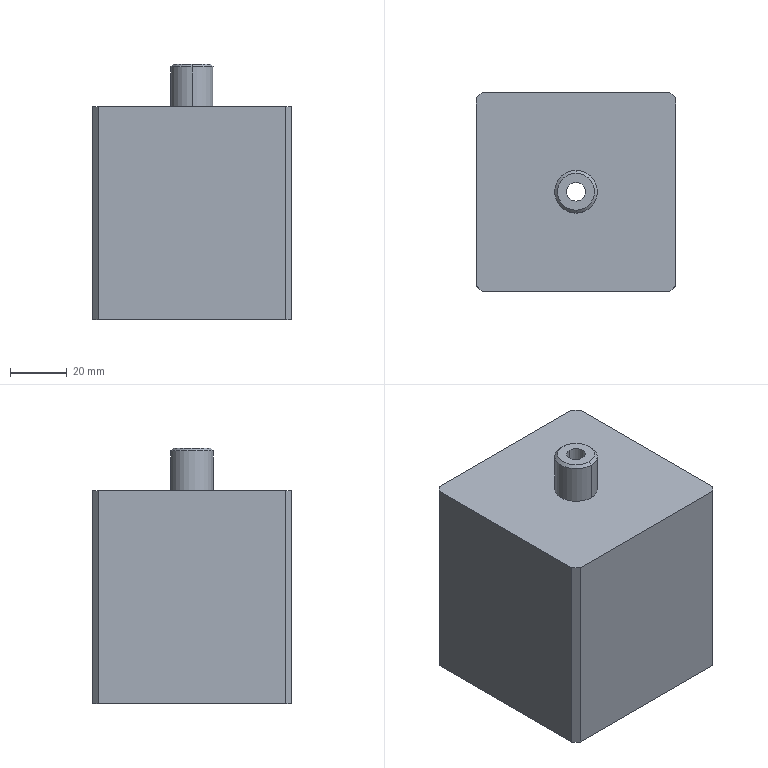NC program | NX | posted with a generic post | part box 70 x 70 x 90 mm
Lines 7860 to 8019 of 10206:
(ZLEVEL_PROFILE_COPY_COPY , TOOL : D10)
N15706 T04 M6
N15708 G54
N15710 G17 G0 G90 X-15.583 Y10.337 S7500 M3
N15712 G43 Z30. H4
N15714 Z-8.214
N15716 G94 G1 Z-9.714 F1000.
N15718 X-17.225 Y10.843
N15720 G3 X-18.2 Y10.62 R1.
N15722 G1 Y-10.62 F850.
N15724 G3 X18.2 Y-10.62 R25.64
N15726 G1 Y10.62
N15728 G3 X-18.2 Y10.62 R25.64
N15730 X-17.7 Y9.754 R1.
N15732 G1 X-16.2 Y8.888
N15734 Z-8.214
N15736 G0 X-15.583 Y10.337 Z-17.929
N15738 G1 Z-19.429 F1000.
N15740 X-17.225 Y10.843
N15742 G3 X-18.2 Y10.62 R1.
N15744 G1 Y-10.62 F850.
N15746 G3 X18.2 Y-10.62 R25.64
N15748 G1 Y10.62
N15750 G3 X-18.2 Y10.62 R25.64
N15752 X-17.7 Y9.754 R1.
N15754 G1 X-16.2 Y8.888
N15756 Z-17.929
N15758 G0 X-15.583 Y10.337 Z-27.643
N15760 G1 Z-29.143 F1000.
N15762 X-17.225 Y10.843
N15764 G3 X-18.2 Y10.62 R1.
N15766 G1 Y-10.621 F850.
N15768 G3 X18.2 Y-10.621 R25.64
N15770 G1 Y10.62
N15772 G3 X-18.2 Y10.62 R25.64
N15774 X-17.7 Y9.754 R1.
N15776 G1 X-16.2 Y8.888
N15778 Z-27.643
N15780 G0 X-15.583 Y10.337 Z-37.357
N15782 G1 Z-38.857 F1000.
N15784 X-17.225 Y10.843
N15786 G3 X-18.2 Y10.62 R1.
N15788 G1 Y-10.621 F850.
N15790 G3 X18.2 Y-10.621 R25.64
N15792 G1 Y10.62
N15794 G3 X-18.2 Y10.62 R25.64
N15796 X-17.7 Y9.754 R1.
N15798 G1 X-16.2 Y8.888
N15800 Z-37.357
N15802 G0 X-15.583 Y10.337 Z-47.071
N15804 G1 Z-48.571 F1000.
N15806 X-17.225 Y10.843
N15808 G3 X-18.2 Y10.62 R1.
N15810 G1 Y-10.621 F850.
N15812 G3 X18.2 Y-10.621 R25.64
N15814 G1 Y10.62
N15816 G3 X-18.2 Y10.62 R25.64
N15818 X-17.7 Y9.754 R1.
N15820 G1 X-16.2 Y8.888
N15822 Z-47.071
N15824 G0 X-15.583 Y10.337 Z-56.786
N15826 G1 Z-58.286 F1000.
N15828 X-17.225 Y10.843
N15830 G3 X-18.2 Y10.62 R1.
N15832 G1 Y-10.621 F850.
N15834 G3 X18.2 Y-10.621 R25.64
N15836 G1 Y10.62
N15838 G3 X-18.2 Y10.62 R25.64
N15840 X-17.7 Y9.754 R1.
N15842 G1 X-16.2 Y8.888
N15844 Z-56.786
N15846 G0 X-15.583 Y10.337 Z-66.5
N15848 G1 Z-68. F1000.
N15850 X-17.225 Y10.843
N15852 G3 X-18.2 Y10.62 R1.
N15854 G1 Y-10.621 F850.
N15856 G3 X18.2 Y-10.621 R25.64
N15858 G1 Y10.62
N15860 G3 X-18.2 Y10.62 R25.64
N15862 X-17.7 Y9.754 R1.
N15864 G1 X-16.2 Y8.888
N15866 Z-66.5
N15868 G0 Z30.
(FLOOR_WALL_1_COPY_COPY , TOOL : D10)
N15870 X-17.197 Y-9.55
N15872 Z-66.5
N15874 G1 Z-68. F1000.
N15876 G3 X-17.697 Y-10.416 R1.
N15878 G1 Y10.416
N15880 G2 X-11.798 Y14.76 R25.14
N15882 G1 Y-14.76
N15884 G3 X-5.898 Y-16.998 R25.14
N15886 G1 Y16.998
N15888 G2 X0.001 Y17.7 R25.14
N15890 G1 Y-17.7
N15892 G3 X5.901 Y-16.998 R25.14
N15894 G1 Y16.998
N15896 G2 X11.8 Y14.758 R25.14
N15898 G1 Y-14.758
N15900 G3 X17.7 Y-10.413 R25.14
N15902 G1 Y10.413
N15904 G3 X16.723 Y10.627 R1.
N15906 G1 X18.184 Y10.286
N15908 G3 X18.052 Y10.768 R0.5
N15910 X-18.2 Y10.62 R25.64
N15912 G1 Y-10.62
N15914 G3 X18.2 Y-10.62 R25.64
N15916 G1 Y10.62
N15918 G3 X18.052 Y10.768 R25.64
N15920 X17.085 Y11.023 R1.
N15922 G1 X15.921 Y10.706
N15924 Z-66.5
N15926 G0 Z30.
N15928 M5
(PLANAR_MILL_COPY_COPY , TOOL : D8A45)
N15930 T06 M6
N15932 G54
N15934 G17 G0 G90 X-40.3 Y0. S7500 M3
N15936 G43 Z30. H6
N15938 Z1.5
N15940 G94 G1 Z-1.5 F1250.
N15942 X-36.3
N15944 Y33.
N15946 G2 X-35.919 Y33.919 R1.3
N15948 G1 X-33.919 Y35.919
N15950 G2 X-33. Y36.3 R1.3
N15952 G1 X33.
N15954 G2 X33.919 Y35.919 R1.3
N15956 G1 X35.919 Y33.919
N15958 G2 X36.3 Y33. R1.3
N15960 G1 Y-33.
N15962 G2 X35.919 Y-33.919 R1.3
N15964 G1 X33.919 Y-35.919
N15966 G2 X33. Y-36.3 R1.3
N15968 G1 X-33.
N15970 G2 X-33.919 Y-35.919 R1.3
N15972 G1 X-35.919 Y-33.919
N15974 G2 X-36.3 Y-33. R1.3
N15976 G1 Y0.
N15978 X-40.3
N15980 Z1.5
N15982 G0 Z30.
N15984 M5
(DRILLING_COPY_1 , TOOL : 14.0ZT)
N15986 T18 M6
N15988 G54
N15990 G17 G0 G90 X0. Y0. S3000 M3
N15992 G43 Z30. H18
N15994 G94 G81 G98 Z-74.4 F250. R-65.
N15996 G80
N15998 G0 X0. Y0. Z30.
N16000 M5